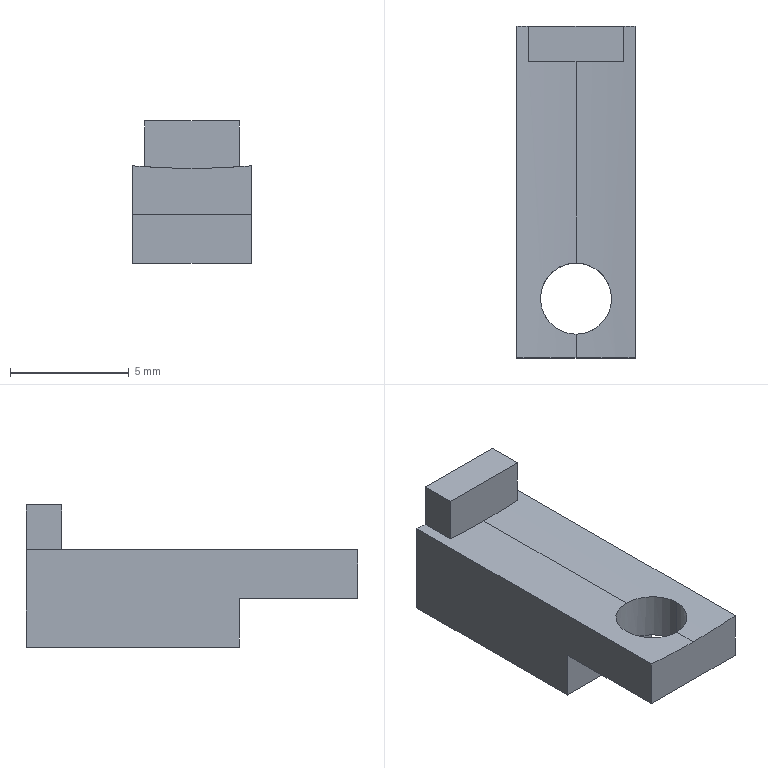Part | STEP file | Guide wheel mechanism revised.sldasm-Part-435 | 1 solid | 15 faces | box 5 x 14 x 6 mm | volume 229.161 mm3 | plane 11 | cylinder 4 | commonest cylinder face diameters 3 x2 60 x2
STEP:
#1=CARTESIAN_POINT('',(0.,1.,-30.));
#2=VERTEX_POINT('',#1);
#3=CARTESIAN_POINT('',(1.5,2.5,-29.962));
#4=VERTEX_POINT('',#3);
#5=CARTESIAN_POINT('',(0.,1.,-30.));
#6=CARTESIAN_POINT('',(0.09783,1.,-30.));
#7=CARTESIAN_POINT('',(0.1972,1.01,-30.));
#8=CARTESIAN_POINT('',(0.3895,1.048,-29.998));
#9=CARTESIAN_POINT('',(0.483,1.077,-29.996));
#10=CARTESIAN_POINT('',(0.6646,1.152,-29.993));
#11=CARTESIAN_POINT('',(0.7524,1.199,-29.991));
#12=CARTESIAN_POINT('',(0.9149,1.307,-29.986));
#13=CARTESIAN_POINT('',(0.9906,1.369,-29.984));
#14=CARTESIAN_POINT('',(1.201,1.579,-29.976));
#15=CARTESIAN_POINT('',(1.311,1.744,-29.971));
#16=CARTESIAN_POINT('',(1.424,2.017,-29.966));
#17=CARTESIAN_POINT('',(1.452,2.111,-29.965));
#18=CARTESIAN_POINT('',(1.49,2.303,-29.963));
#19=CARTESIAN_POINT('',(1.5,2.402,-29.962));
#20=CARTESIAN_POINT('',(1.5,2.5,-29.962));
#21=B_SPLINE_CURVE_WITH_KNOTS('',3,(#5,#6,#7,#8,#9,#10,#11,#12,#13,#14,#15,#16,#17,#18,#19,#20),.UNSPECIFIED.,.F.,.F.,(4,2,2,2,2,2,2,4),(0.002346,0.002639,0.002932,0.003225,0.003518,0.004104,0.004397,0.00469),.UNSPECIFIED.);
#22=EDGE_CURVE('',#2,#4,#21,.T.);
#23=ORIENTED_EDGE('',*,*,#22,.T.);
#24=CARTESIAN_POINT('',(1.5,2.5,-31.948));
#25=VERTEX_POINT('',#24);
#26=CARTESIAN_POINT('',(1.5,2.5,-27.999));
#27=DIRECTION('',(0.,0.,-1.));
#28=VECTOR('',#27,1000.);
#29=LINE('',#26,#28);
#30=EDGE_CURVE('',#4,#25,#29,.T.);
#31=ORIENTED_EDGE('',*,*,#30,.T.);
#32=CARTESIAN_POINT('',(-1.5,2.5,-31.948));
#33=VERTEX_POINT('',#32);
#34=CARTESIAN_POINT('',(0.,2.5,-31.948));
#35=DIRECTION('',(0.,0.,-1.));
#36=DIRECTION('',(-1.,0.,0.));
#37=AXIS2_PLACEMENT_3D('',#34,#35,#36);
#38=CIRCLE('',#37,1.5);
#39=EDGE_CURVE('',#25,#33,#38,.T.);
#40=ORIENTED_EDGE('',*,*,#39,.T.);
#41=CARTESIAN_POINT('',(-1.5,2.5,-29.962));
#42=VERTEX_POINT('',#41);
#43=CARTESIAN_POINT('',(-1.5,2.5,-27.999));
#44=DIRECTION('',(0.,0.,-1.));
#45=VECTOR('',#44,1000.);
#46=LINE('',#43,#45);
#47=EDGE_CURVE('',#42,#33,#46,.T.);
#48=ORIENTED_EDGE('',*,*,#47,.F.);
#49=CARTESIAN_POINT('',(-1.5,2.5,-29.962));
#50=CARTESIAN_POINT('',(-1.5,2.401,-29.962));
#51=CARTESIAN_POINT('',(-1.49,2.303,-29.963));
#52=CARTESIAN_POINT('',(-1.452,2.112,-29.965));
#53=CARTESIAN_POINT('',(-1.423,2.016,-29.966));
#54=CARTESIAN_POINT('',(-1.348,1.835,-29.97));
#55=CARTESIAN_POINT('',(-1.302,1.748,-29.972));
#56=CARTESIAN_POINT('',(-1.193,1.585,-29.976));
#57=CARTESIAN_POINT('',(-1.13,1.508,-29.979));
#58=CARTESIAN_POINT('',(-0.9218,1.301,-29.986));
#59=CARTESIAN_POINT('',(-0.7544,1.189,-29.991));
#60=CARTESIAN_POINT('',(-0.3932,1.039,-29.998));
#61=CARTESIAN_POINT('',(-0.1958,1.,-30.));
#62=CARTESIAN_POINT('',(0.,1.,-30.));
#63=B_SPLINE_CURVE_WITH_KNOTS('',3,(#49,#50,#51,#52,#53,#54,#55,#56,#57,#58,#59,#60,#61,#62),.UNSPECIFIED.,.F.,.F.,(4,2,2,2,2,2,4),(0.,0.0002932,0.0005864,0.0008797,0.001173,0.001759,0.002346),.UNSPECIFIED.);
#64=EDGE_CURVE('',#42,#2,#63,.T.);
#65=ORIENTED_EDGE('',*,*,#64,.T.);
#66=EDGE_LOOP('',(#23,#31,#40,#48,#65));
#67=FACE_OUTER_BOUND('',#66,.T.);
#68=CARTESIAN_POINT('',(0.,2.5,-27.999));
#69=DIRECTION('',(0.,0.,-1.));
#70=DIRECTION('',(-1.,0.,0.));
#71=AXIS2_PLACEMENT_3D('',#68,#69,#70);
#72=CYLINDRICAL_SURFACE('',#71,1.5);
#73=ADVANCED_FACE('',(#67),#72,.F.);
#74=CARTESIAN_POINT('',(0.,12.5,-30.));
#75=VERTEX_POINT('',#74);
#76=CARTESIAN_POINT('',(2.,12.5,-29.933));
#77=VERTEX_POINT('',#76);
#78=CARTESIAN_POINT('',(0.,12.5,0.));
#79=DIRECTION('',(0.,-1.,0.));
#80=DIRECTION('',(0.,0.,1.));
#81=AXIS2_PLACEMENT_3D('',#78,#79,#80);
#82=CIRCLE('',#81,30.);
#83=EDGE_CURVE('',#75,#77,#82,.T.);
#84=ORIENTED_EDGE('',*,*,#83,.F.);
#85=CARTESIAN_POINT('',(0.,4.,-30.));
#86=VERTEX_POINT('',#85);
#87=CARTESIAN_POINT('',(0.,14.,-30.));
#88=DIRECTION('',(0.,-1.,0.));
#89=VECTOR('',#88,1000.);
#90=LINE('',#87,#89);
#91=EDGE_CURVE('',#75,#86,#90,.T.);
#92=ORIENTED_EDGE('',*,*,#91,.T.);
#93=CARTESIAN_POINT('',(1.5,2.5,-29.962));
#94=CARTESIAN_POINT('',(1.5,2.696,-29.962));
#95=CARTESIAN_POINT('',(1.461,2.893,-29.965));
#96=CARTESIAN_POINT('',(1.311,3.254,-29.971));
#97=CARTESIAN_POINT('',(1.199,3.422,-29.976));
#98=CARTESIAN_POINT('',(0.9918,3.63,-29.984));
#99=CARTESIAN_POINT('',(0.9147,3.693,-29.986));
#100=CARTESIAN_POINT('',(0.7515,3.802,-29.991));
#101=CARTESIAN_POINT('',(0.6653,3.848,-29.993));
#102=CARTESIAN_POINT('',(0.4837,3.923,-29.996));
#103=CARTESIAN_POINT('',(0.3883,3.952,-29.998));
#104=CARTESIAN_POINT('',(0.1964,3.99,-30.));
#105=CARTESIAN_POINT('',(0.09901,4.,-30.));
#106=CARTESIAN_POINT('',(0.,4.,-30.));
#107=B_SPLINE_CURVE_WITH_KNOTS('',3,(#93,#94,#95,#96,#97,#98,#99,#100,#101,#102,#103,#104,#105,#106),.UNSPECIFIED.,.F.,.F.,(4,2,2,2,2,2,4),(0.00469,0.005277,0.005863,0.006157,0.00645,0.006743,0.007036),.UNSPECIFIED.);
#108=EDGE_CURVE('',#4,#86,#107,.T.);
#109=ORIENTED_EDGE('',*,*,#108,.F.);
#110=ORIENTED_EDGE('',*,*,#22,.F.);
#111=CARTESIAN_POINT('',(0.,0.,-30.));
#112=VERTEX_POINT('',#111);
#113=CARTESIAN_POINT('',(0.,14.,-30.));
#114=DIRECTION('',(0.,-1.,0.));
#115=VECTOR('',#114,1000.);
#116=LINE('',#113,#115);
#117=EDGE_CURVE('',#2,#112,#116,.T.);
#118=ORIENTED_EDGE('',*,*,#117,.T.);
#119=CARTESIAN_POINT('',(2.5,0.,-29.896));
#120=VERTEX_POINT('',#119);
#121=CARTESIAN_POINT('',(0.,0.,0.));
#122=DIRECTION('',(0.,-1.,0.));
#123=DIRECTION('',(0.,0.,1.));
#124=AXIS2_PLACEMENT_3D('',#121,#122,#123);
#125=CIRCLE('',#124,30.);
#126=EDGE_CURVE('',#112,#120,#125,.T.);
#127=ORIENTED_EDGE('',*,*,#126,.T.);
#128=CARTESIAN_POINT('',(2.5,14.,-29.896));
#129=VERTEX_POINT('',#128);
#130=CARTESIAN_POINT('',(2.5,14.,-29.896));
#131=DIRECTION('',(0.,-1.,0.));
#132=VECTOR('',#131,1000.);
#133=LINE('',#130,#132);
#134=EDGE_CURVE('',#129,#120,#133,.T.);
#135=ORIENTED_EDGE('',*,*,#134,.F.);
#136=CARTESIAN_POINT('',(2.,14.,-29.933));
#137=VERTEX_POINT('',#136);
#138=CARTESIAN_POINT('',(0.,14.,0.));
#139=DIRECTION('',(0.,-1.,0.));
#140=DIRECTION('',(0.,0.,1.));
#141=AXIS2_PLACEMENT_3D('',#138,#139,#140);
#142=CIRCLE('',#141,30.);
#143=EDGE_CURVE('',#137,#129,#142,.T.);
#144=ORIENTED_EDGE('',*,*,#143,.F.);
#145=CARTESIAN_POINT('',(2.,14.,-29.933));
#146=DIRECTION('',(0.,-1.,0.));
#147=VECTOR('',#146,1000.);
#148=LINE('',#145,#147);
#149=EDGE_CURVE('',#137,#77,#148,.T.);
#150=ORIENTED_EDGE('',*,*,#149,.T.);
#151=EDGE_LOOP('',(#84,#92,#109,#110,#118,#127,#135,#144,#150));
#152=FACE_OUTER_BOUND('',#151,.T.);
#153=CARTESIAN_POINT('',(0.,14.,0.));
#154=DIRECTION('',(0.,-1.,0.));
#155=DIRECTION('',(0.,0.,-1.));
#156=AXIS2_PLACEMENT_3D('',#153,#154,#155);
#157=CYLINDRICAL_SURFACE('',#156,30.);
#158=ADVANCED_FACE('',(#152),#157,.F.);
#159=CARTESIAN_POINT('',(-2.5,5.,-34.));
#160=VERTEX_POINT('',#159);
#161=CARTESIAN_POINT('',(2.5,5.,-34.));
#162=VERTEX_POINT('',#161);
#163=CARTESIAN_POINT('',(-2.5,5.,-34.));
#164=DIRECTION('',(1.,0.,0.));
#165=VECTOR('',#164,1000.);
#166=LINE('',#163,#165);
#167=EDGE_CURVE('',#160,#162,#166,.T.);
#168=ORIENTED_EDGE('',*,*,#167,.F.);
#169=CARTESIAN_POINT('',(-2.5,14.,-34.));
#170=VERTEX_POINT('',#169);
#171=CARTESIAN_POINT('',(-2.5,14.,-34.));
#172=DIRECTION('',(0.,-1.,0.));
#173=VECTOR('',#172,1000.);
#174=LINE('',#171,#173);
#175=EDGE_CURVE('',#170,#160,#174,.T.);
#176=ORIENTED_EDGE('',*,*,#175,.F.);
#177=CARTESIAN_POINT('',(2.5,14.,-34.));
#178=VERTEX_POINT('',#177);
#179=CARTESIAN_POINT('',(-2.5,14.,-34.));
#180=DIRECTION('',(-1.,0.,0.));
#181=VECTOR('',#180,1000.);
#182=LINE('',#179,#181);
#183=EDGE_CURVE('',#178,#170,#182,.T.);
#184=ORIENTED_EDGE('',*,*,#183,.F.);
#185=CARTESIAN_POINT('',(2.5,14.,-34.));
#186=DIRECTION('',(0.,-1.,0.));
#187=VECTOR('',#186,1000.);
#188=LINE('',#185,#187);
#189=EDGE_CURVE('',#178,#162,#188,.T.);
#190=ORIENTED_EDGE('',*,*,#189,.T.);
#191=EDGE_LOOP('',(#168,#176,#184,#190));
#192=FACE_OUTER_BOUND('',#191,.T.);
#193=CARTESIAN_POINT('',(-2.5,14.,-34.));
#194=DIRECTION('',(0.,0.,1.));
#195=DIRECTION('',(1.,0.,0.));
#196=AXIS2_PLACEMENT_3D('',#193,#194,#195);
#197=PLANE('',#196);
#198=ADVANCED_FACE('',(#192),#197,.F.);
#199=ORIENTED_EDGE('',*,*,#91,.F.);
#200=CARTESIAN_POINT('',(-2.,12.5,-29.933));
#201=VERTEX_POINT('',#200);
#202=CARTESIAN_POINT('',(0.,12.5,0.));
#203=DIRECTION('',(0.,-1.,0.));
#204=DIRECTION('',(0.,0.,1.));
#205=AXIS2_PLACEMENT_3D('',#202,#203,#204);
#206=CIRCLE('',#205,30.);
#207=EDGE_CURVE('',#201,#75,#206,.T.);
#208=ORIENTED_EDGE('',*,*,#207,.F.);
#209=CARTESIAN_POINT('',(-2.,14.,-29.933));
#210=VERTEX_POINT('',#209);
#211=CARTESIAN_POINT('',(-2.,14.,-29.933));
#212=DIRECTION('',(0.,1.,0.));
#213=VECTOR('',#212,1000.);
#214=LINE('',#211,#213);
#215=EDGE_CURVE('',#201,#210,#214,.T.);
#216=ORIENTED_EDGE('',*,*,#215,.T.);
#217=CARTESIAN_POINT('',(-2.5,14.,-29.896));
#218=VERTEX_POINT('',#217);
#219=CARTESIAN_POINT('',(0.,14.,0.));
#220=DIRECTION('',(0.,-1.,0.));
#221=DIRECTION('',(0.,0.,1.));
#222=AXIS2_PLACEMENT_3D('',#219,#220,#221);
#223=CIRCLE('',#222,30.);
#224=EDGE_CURVE('',#218,#210,#223,.T.);
#225=ORIENTED_EDGE('',*,*,#224,.F.);
#226=CARTESIAN_POINT('',(-2.5,0.,-29.896));
#227=VERTEX_POINT('',#226);
#228=CARTESIAN_POINT('',(-2.5,14.,-29.896));
#229=DIRECTION('',(0.,-1.,0.));
#230=VECTOR('',#229,1000.);
#231=LINE('',#228,#230);
#232=EDGE_CURVE('',#218,#227,#231,.T.);
#233=ORIENTED_EDGE('',*,*,#232,.T.);
#234=CARTESIAN_POINT('',(0.,0.,0.));
#235=DIRECTION('',(0.,-1.,0.));
#236=DIRECTION('',(0.,0.,1.));
#237=AXIS2_PLACEMENT_3D('',#234,#235,#236);
#238=CIRCLE('',#237,30.);
#239=EDGE_CURVE('',#227,#112,#238,.T.);
#240=ORIENTED_EDGE('',*,*,#239,.T.);
#241=ORIENTED_EDGE('',*,*,#117,.F.);
#242=ORIENTED_EDGE('',*,*,#64,.F.);
#243=CARTESIAN_POINT('',(0.,4.,-30.));
#244=CARTESIAN_POINT('',(-0.1978,4.,-30.));
#245=CARTESIAN_POINT('',(-0.3924,3.961,-29.998));
#246=CARTESIAN_POINT('',(-0.665,3.848,-29.993));
#247=CARTESIAN_POINT('',(-0.7511,3.802,-29.991));
#248=CARTESIAN_POINT('',(-0.914,3.693,-29.986));
#249=CARTESIAN_POINT('',(-0.9911,3.63,-29.984));
#250=CARTESIAN_POINT('',(-1.199,3.423,-29.976));
#251=CARTESIAN_POINT('',(-1.31,3.256,-29.971));
#252=CARTESIAN_POINT('',(-1.46,2.895,-29.965));
#253=CARTESIAN_POINT('',(-1.5,2.698,-29.962));
#254=CARTESIAN_POINT('',(-1.5,2.5,-29.962));
#255=B_SPLINE_CURVE_WITH_KNOTS('',3,(#243,#244,#245,#246,#247,#248,#249,#250,#251,#252,#253,#254),.UNSPECIFIED.,.F.,.F.,(4,2,2,2,2,4),(0.007036,0.007622,0.007915,0.008208,0.008794,0.00938),.UNSPECIFIED.);
#256=EDGE_CURVE('',#86,#42,#255,.T.);
#257=ORIENTED_EDGE('',*,*,#256,.F.);
#258=EDGE_LOOP('',(#199,#208,#216,#225,#233,#240,#241,#242,#257));
#259=FACE_OUTER_BOUND('',#258,.T.);
#260=CARTESIAN_POINT('',(0.,14.,0.));
#261=DIRECTION('',(0.,-1.,0.));
#262=DIRECTION('',(0.,0.,-1.));
#263=AXIS2_PLACEMENT_3D('',#260,#261,#262);
#264=CYLINDRICAL_SURFACE('',#263,30.);
#265=ADVANCED_FACE('',(#259),#264,.F.);
#266=CARTESIAN_POINT('',(2.5,0.,-31.948));
#267=VERTEX_POINT('',#266);
#268=CARTESIAN_POINT('',(2.5,0.,-34.));
#269=DIRECTION('',(0.,0.,-1.));
#270=VECTOR('',#269,1000.);
#271=LINE('',#268,#270);
#272=EDGE_CURVE('',#120,#267,#271,.T.);
#273=ORIENTED_EDGE('',*,*,#272,.T.);
#274=CARTESIAN_POINT('',(2.5,5.,-31.948));
#275=VERTEX_POINT('',#274);
#276=CARTESIAN_POINT('',(2.5,5.,-31.948));
#277=DIRECTION('',(0.,-1.,0.));
#278=VECTOR('',#277,1000.);
#279=LINE('',#276,#278);
#280=EDGE_CURVE('',#275,#267,#279,.T.);
#281=ORIENTED_EDGE('',*,*,#280,.F.);
#282=CARTESIAN_POINT('',(2.5,5.,-31.948));
#283=DIRECTION('',(0.,0.,1.));
#284=VECTOR('',#283,1000.);
#285=LINE('',#282,#284);
#286=EDGE_CURVE('',#162,#275,#285,.T.);
#287=ORIENTED_EDGE('',*,*,#286,.F.);
#288=ORIENTED_EDGE('',*,*,#189,.F.);
#289=CARTESIAN_POINT('',(2.5,14.,-34.));
#290=DIRECTION('',(0.,0.,-1.));
#291=VECTOR('',#290,1000.);
#292=LINE('',#289,#291);
#293=EDGE_CURVE('',#129,#178,#292,.T.);
#294=ORIENTED_EDGE('',*,*,#293,.F.);
#295=ORIENTED_EDGE('',*,*,#134,.T.);
#296=EDGE_LOOP('',(#273,#281,#287,#288,#294,#295));
#297=FACE_OUTER_BOUND('',#296,.T.);
#298=CARTESIAN_POINT('',(2.5,14.,-34.));
#299=DIRECTION('',(-1.,0.,0.));
#300=DIRECTION('',(0.,0.,1.));
#301=AXIS2_PLACEMENT_3D('',#298,#299,#300);
#302=PLANE('',#301);
#303=ADVANCED_FACE('',(#297),#302,.F.);
#304=CARTESIAN_POINT('',(-2.5,5.,-31.948));
#305=VERTEX_POINT('',#304);
#306=CARTESIAN_POINT('',(-2.5,5.,-31.948));
#307=DIRECTION('',(0.,0.,-1.));
#308=VECTOR('',#307,1000.);
#309=LINE('',#306,#308);
#310=EDGE_CURVE('',#305,#160,#309,.T.);
#311=ORIENTED_EDGE('',*,*,#310,.F.);
#312=CARTESIAN_POINT('',(-2.5,0.,-31.948));
#313=VERTEX_POINT('',#312);
#314=CARTESIAN_POINT('',(-2.5,5.,-31.948));
#315=DIRECTION('',(0.,-1.,0.));
#316=VECTOR('',#315,1000.);
#317=LINE('',#314,#316);
#318=EDGE_CURVE('',#305,#313,#317,.T.);
#319=ORIENTED_EDGE('',*,*,#318,.T.);
#320=CARTESIAN_POINT('',(-2.5,0.,-34.));
#321=DIRECTION('',(0.,0.,1.));
#322=VECTOR('',#321,1000.);
#323=LINE('',#320,#322);
#324=EDGE_CURVE('',#313,#227,#323,.T.);
#325=ORIENTED_EDGE('',*,*,#324,.T.);
#326=ORIENTED_EDGE('',*,*,#232,.F.);
#327=CARTESIAN_POINT('',(-2.5,14.,-34.));
#328=DIRECTION('',(0.,0.,1.));
#329=VECTOR('',#328,1000.);
#330=LINE('',#327,#329);
#331=EDGE_CURVE('',#170,#218,#330,.T.);
#332=ORIENTED_EDGE('',*,*,#331,.F.);
#333=ORIENTED_EDGE('',*,*,#175,.T.);
#334=EDGE_LOOP('',(#311,#319,#325,#326,#332,#333));
#335=FACE_OUTER_BOUND('',#334,.T.);
#336=CARTESIAN_POINT('',(-2.5,14.,-34.));
#337=DIRECTION('',(1.,0.,0.));
#338=DIRECTION('',(0.,0.,-1.));
#339=AXIS2_PLACEMENT_3D('',#336,#337,#338);
#340=PLANE('',#339);
#341=ADVANCED_FACE('',(#335),#340,.F.);
#342=ORIENTED_EDGE('',*,*,#183,.T.);
#343=ORIENTED_EDGE('',*,*,#331,.T.);
#344=ORIENTED_EDGE('',*,*,#224,.T.);
#345=CARTESIAN_POINT('',(-2.,14.,-28.));
#346=VERTEX_POINT('',#345);
#347=CARTESIAN_POINT('',(-2.,14.,-34.));
#348=DIRECTION('',(0.,0.,1.));
#349=VECTOR('',#348,1000.);
#350=LINE('',#347,#349);
#351=EDGE_CURVE('',#210,#346,#350,.T.);
#352=ORIENTED_EDGE('',*,*,#351,.T.);
#353=CARTESIAN_POINT('',(2.,14.,-28.));
#354=VERTEX_POINT('',#353);
#355=CARTESIAN_POINT('',(-2.,14.,-28.));
#356=DIRECTION('',(1.,0.,0.));
#357=VECTOR('',#356,1000.);
#358=LINE('',#355,#357);
#359=EDGE_CURVE('',#346,#354,#358,.T.);
#360=ORIENTED_EDGE('',*,*,#359,.T.);
#361=CARTESIAN_POINT('',(2.,14.,-34.));
#362=DIRECTION('',(0.,0.,-1.));
#363=VECTOR('',#362,1000.);
#364=LINE('',#361,#363);
#365=EDGE_CURVE('',#354,#137,#364,.T.);
#366=ORIENTED_EDGE('',*,*,#365,.T.);
#367=ORIENTED_EDGE('',*,*,#143,.T.);
#368=ORIENTED_EDGE('',*,*,#293,.T.);
#369=EDGE_LOOP('',(#342,#343,#344,#352,#360,#366,#367,#368));
#370=FACE_OUTER_BOUND('',#369,.T.);
#371=CARTESIAN_POINT('',(0.,14.,0.));
#372=DIRECTION('',(0.,1.,0.));
#373=DIRECTION('',(0.,0.,1.));
#374=AXIS2_PLACEMENT_3D('',#371,#372,#373);
#375=PLANE('',#374);
#376=ADVANCED_FACE('',(#370),#375,.T.);
#377=ORIENTED_EDGE('',*,*,#324,.F.);
#378=CARTESIAN_POINT('',(-2.5,0.,-31.948));
#379=DIRECTION('',(-1.,0.,0.));
#380=VECTOR('',#379,1000.);
#381=LINE('',#378,#380);
#382=EDGE_CURVE('',#267,#313,#381,.T.);
#383=ORIENTED_EDGE('',*,*,#382,.F.);
#384=ORIENTED_EDGE('',*,*,#272,.F.);
#385=ORIENTED_EDGE('',*,*,#126,.F.);
#386=ORIENTED_EDGE('',*,*,#239,.F.);
#387=EDGE_LOOP('',(#377,#383,#384,#385,#386));
#388=FACE_OUTER_BOUND('',#387,.T.);
#389=CARTESIAN_POINT('',(0.,0.,0.));
#390=DIRECTION('',(0.,1.,0.));
#391=DIRECTION('',(0.,0.,1.));
#392=AXIS2_PLACEMENT_3D('',#389,#390,#391);
#393=PLANE('',#392);
#394=ADVANCED_FACE('',(#388),#393,.F.);
#395=CARTESIAN_POINT('',(-2.,12.5,-28.));
#396=VERTEX_POINT('',#395);
#397=CARTESIAN_POINT('',(-2.,12.5,-34.));
#398=DIRECTION('',(0.,0.,1.));
#399=VECTOR('',#398,1000.);
#400=LINE('',#397,#399);
#401=EDGE_CURVE('',#201,#396,#400,.T.);
#402=ORIENTED_EDGE('',*,*,#401,.F.);
#403=ORIENTED_EDGE('',*,*,#207,.T.);
#404=ORIENTED_EDGE('',*,*,#83,.T.);
#405=CARTESIAN_POINT('',(2.,12.5,-28.));
#406=VERTEX_POINT('',#405);
#407=CARTESIAN_POINT('',(2.,12.5,-34.));
#408=DIRECTION('',(0.,0.,-1.));
#409=VECTOR('',#408,1000.);
#410=LINE('',#407,#409);
#411=EDGE_CURVE('',#406,#77,#410,.T.);
#412=ORIENTED_EDGE('',*,*,#411,.F.);
#413=CARTESIAN_POINT('',(-2.,12.5,-28.));
#414=DIRECTION('',(1.,0.,0.));
#415=VECTOR('',#414,1000.);
#416=LINE('',#413,#415);
#417=EDGE_CURVE('',#396,#406,#416,.T.);
#418=ORIENTED_EDGE('',*,*,#417,.F.);
#419=EDGE_LOOP('',(#402,#403,#404,#412,#418));
#420=FACE_OUTER_BOUND('',#419,.T.);
#421=CARTESIAN_POINT('',(0.,12.5,0.));
#422=DIRECTION('',(0.,1.,0.));
#423=DIRECTION('',(0.,0.,1.));
#424=AXIS2_PLACEMENT_3D('',#421,#422,#423);
#425=PLANE('',#424);
#426=ADVANCED_FACE('',(#420),#425,.F.);
#427=ORIENTED_EDGE('',*,*,#215,.F.);
#428=ORIENTED_EDGE('',*,*,#401,.T.);
#429=CARTESIAN_POINT('',(-2.,12.5,-28.));
#430=DIRECTION('',(0.,1.,0.));
#431=VECTOR('',#430,1000.);
#432=LINE('',#429,#431);
#433=EDGE_CURVE('',#396,#346,#432,.T.);
#434=ORIENTED_EDGE('',*,*,#433,.T.);
#435=ORIENTED_EDGE('',*,*,#351,.F.);
#436=EDGE_LOOP('',(#427,#428,#434,#435));
#437=FACE_OUTER_BOUND('',#436,.T.);
#438=CARTESIAN_POINT('',(-2.,12.5,-34.));
#439=DIRECTION('',(-1.,0.,0.));
#440=DIRECTION('',(0.,0.,1.));
#441=AXIS2_PLACEMENT_3D('',#438,#439,#440);
#442=PLANE('',#441);
#443=ADVANCED_FACE('',(#437),#442,.T.);
#444=ORIENTED_EDGE('',*,*,#149,.F.);
#445=ORIENTED_EDGE('',*,*,#365,.F.);
#446=CARTESIAN_POINT('',(2.,12.5,-28.));
#447=DIRECTION('',(0.,1.,0.));
#448=VECTOR('',#447,1000.);
#449=LINE('',#446,#448);
#450=EDGE_CURVE('',#406,#354,#449,.T.);
#451=ORIENTED_EDGE('',*,*,#450,.F.);
#452=ORIENTED_EDGE('',*,*,#411,.T.);
#453=EDGE_LOOP('',(#444,#445,#451,#452));
#454=FACE_OUTER_BOUND('',#453,.T.);
#455=CARTESIAN_POINT('',(2.,12.5,-34.));
#456=DIRECTION('',(1.,0.,0.));
#457=DIRECTION('',(0.,0.,-1.));
#458=AXIS2_PLACEMENT_3D('',#455,#456,#457);
#459=PLANE('',#458);
#460=ADVANCED_FACE('',(#454),#459,.T.);
#461=ORIENTED_EDGE('',*,*,#359,.F.);
#462=ORIENTED_EDGE('',*,*,#433,.F.);
#463=ORIENTED_EDGE('',*,*,#417,.T.);
#464=ORIENTED_EDGE('',*,*,#450,.T.);
#465=EDGE_LOOP('',(#461,#462,#463,#464));
#466=FACE_OUTER_BOUND('',#465,.T.);
#467=CARTESIAN_POINT('',(-2.,12.5,-28.));
#468=DIRECTION('',(0.,0.,1.));
#469=DIRECTION('',(1.,0.,0.));
#470=AXIS2_PLACEMENT_3D('',#467,#468,#469);
#471=PLANE('',#470);
#472=ADVANCED_FACE('',(#466),#471,.T.);
#473=CARTESIAN_POINT('',(0.,2.5,-31.948));
#474=DIRECTION('',(0.,0.,-1.));
#475=DIRECTION('',(-1.,0.,0.));
#476=AXIS2_PLACEMENT_3D('',#473,#474,#475);
#477=CIRCLE('',#476,1.5);
#478=EDGE_CURVE('',#33,#25,#477,.T.);
#479=ORIENTED_EDGE('',*,*,#478,.F.);
#480=ORIENTED_EDGE('',*,*,#39,.F.);
#481=EDGE_LOOP('',(#479,#480));
#482=FACE_BOUND('',#481,.T.);
#483=ORIENTED_EDGE('',*,*,#382,.T.);
#484=ORIENTED_EDGE('',*,*,#318,.F.);
#485=CARTESIAN_POINT('',(-2.5,5.,-31.948));
#486=DIRECTION('',(-1.,0.,0.));
#487=VECTOR('',#486,1000.);
#488=LINE('',#485,#487);
#489=EDGE_CURVE('',#275,#305,#488,.T.);
#490=ORIENTED_EDGE('',*,*,#489,.F.);
#491=ORIENTED_EDGE('',*,*,#280,.T.);
#492=EDGE_LOOP('',(#483,#484,#490,#491));
#493=FACE_OUTER_BOUND('',#492,.T.);
#494=CARTESIAN_POINT('',(-2.5,5.,-31.948));
#495=DIRECTION('',(0.,0.,1.));
#496=DIRECTION('',(1.,0.,0.));
#497=AXIS2_PLACEMENT_3D('',#494,#495,#496);
#498=PLANE('',#497);
#499=ADVANCED_FACE('',(#482,#493),#498,.F.);
#500=ORIENTED_EDGE('',*,*,#310,.T.);
#501=ORIENTED_EDGE('',*,*,#167,.T.);
#502=ORIENTED_EDGE('',*,*,#286,.T.);
#503=ORIENTED_EDGE('',*,*,#489,.T.);
#504=EDGE_LOOP('',(#500,#501,#502,#503));
#505=FACE_OUTER_BOUND('',#504,.T.);
#506=CARTESIAN_POINT('',(0.,5.,0.));
#507=DIRECTION('',(0.,-1.,0.));
#508=DIRECTION('',(0.,0.,-1.));
#509=AXIS2_PLACEMENT_3D('',#506,#507,#508);
#510=PLANE('',#509);
#511=ADVANCED_FACE('',(#505),#510,.T.);
#512=ORIENTED_EDGE('',*,*,#30,.F.);
#513=ORIENTED_EDGE('',*,*,#108,.T.);
#514=ORIENTED_EDGE('',*,*,#256,.T.);
#515=ORIENTED_EDGE('',*,*,#47,.T.);
#516=ORIENTED_EDGE('',*,*,#478,.T.);
#517=EDGE_LOOP('',(#512,#513,#514,#515,#516));
#518=FACE_OUTER_BOUND('',#517,.T.);
#519=CARTESIAN_POINT('',(0.,2.5,-27.999));
#520=DIRECTION('',(0.,0.,-1.));
#521=DIRECTION('',(-1.,0.,0.));
#522=AXIS2_PLACEMENT_3D('',#519,#520,#521);
#523=CYLINDRICAL_SURFACE('',#522,1.5);
#524=ADVANCED_FACE('',(#518),#523,.F.);
#525=CLOSED_SHELL('',(#73,#158,#198,#265,#303,#341,#376,#394,#426,#443,#460,#472,#499,#511,#524));
#526=MANIFOLD_SOLID_BREP('',#525);
#527=CARTESIAN_POINT('',(0.,0.,0.));
#528=DIRECTION('',(0.,0.,1.));
#529=DIRECTION('',(1.,0.,0.));
#530=AXIS2_PLACEMENT_3D('',#527,#528,#529);
#531=(LENGTH_UNIT()NAMED_UNIT(*)SI_UNIT(.MILLI.,.METRE.));
#532=UNCERTAINTY_MEASURE_WITH_UNIT(LENGTH_MEASURE(0.00001),#531,'','');
#533=(NAMED_UNIT(*)PLANE_ANGLE_UNIT()SI_UNIT($,.RADIAN.));
#534=(NAMED_UNIT(*)SI_UNIT($,.STERADIAN.)SOLID_ANGLE_UNIT());
#535=(GEOMETRIC_REPRESENTATION_CONTEXT(3)GLOBAL_UNCERTAINTY_ASSIGNED_CONTEXT((#532))GLOBAL_UNIT_ASSIGNED_CONTEXT((#531,#533,#534))REPRESENTATION_CONTEXT('',''));
#536=ADVANCED_BREP_SHAPE_REPRESENTATION('',(#526,#530),#535);